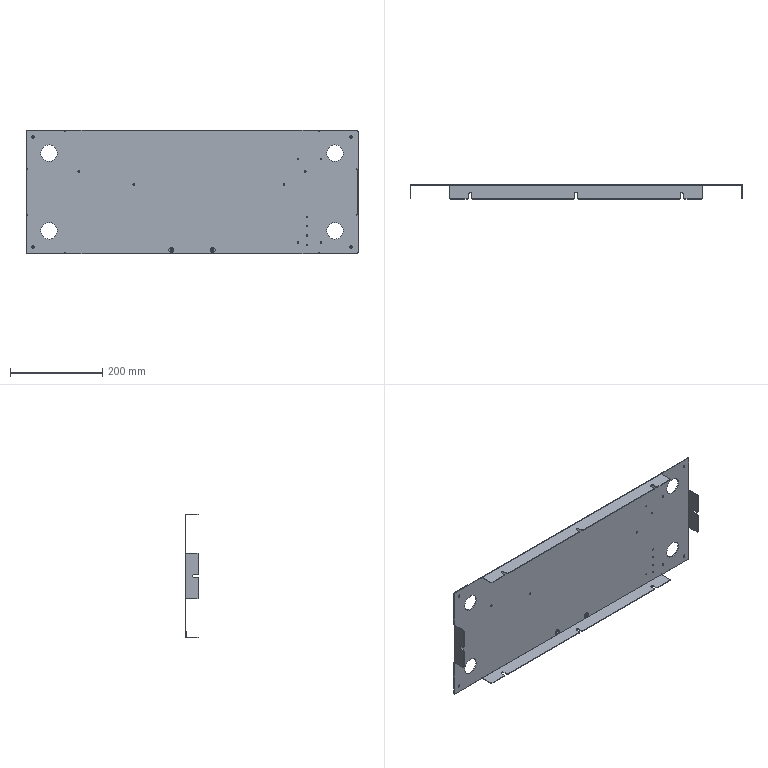Part | STEP file | Cabinet lower base plate | 1 solid | 188 faces | box 718 x 30 x 268 mm | volume 336091 mm3 | cylinder 100 | plane 88 | commonest cylinder face diameters 6 x20 3.3 x16 7 x16 5 x12 2.5 x8 4 x8